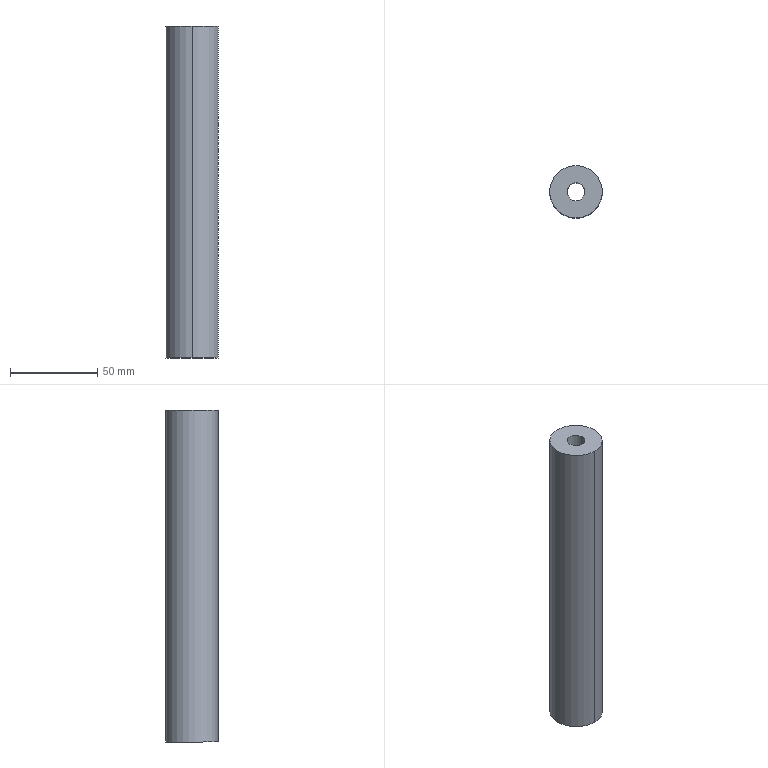Part | SolidWorks | features BaseBody 1 | 1 solid | 6 faces | box 30 x 30 x 190 mm | volume 118778 mm3 | cylinder 4 | plane 2 | commonest cylinder face diameters 10.2 x2 30 x2
STEP:
#1=CARTESIAN_POINT('',(5.1,0.,0.));
#2=VERTEX_POINT('',#1);
#3=CARTESIAN_POINT('',(-5.1,0.,0.));
#4=VERTEX_POINT('',#3);
#5=CARTESIAN_POINT('',(0.,0.,0.));
#6=DIRECTION('',(0.,0.,-1.));
#7=DIRECTION('',(1.,0.,0.));
#8=AXIS2_PLACEMENT_3D('',#5,#6,#7);
#9=CIRCLE('',#8,5.1);
#10=EDGE_CURVE('',#2,#4,#9,.T.);
#11=ORIENTED_EDGE('',*,*,#10,.T.);
#12=CARTESIAN_POINT('',(-5.1,0.,190.));
#13=VERTEX_POINT('',#12);
#14=CARTESIAN_POINT('',(-5.1,0.,0.));
#15=DIRECTION('',(0.,0.,1.));
#16=VECTOR('',#15,1000.);
#17=LINE('',#14,#16);
#18=EDGE_CURVE('',#4,#13,#17,.T.);
#19=ORIENTED_EDGE('',*,*,#18,.T.);
#20=CARTESIAN_POINT('',(5.1,0.,190.));
#21=VERTEX_POINT('',#20);
#22=CARTESIAN_POINT('',(0.,0.,190.));
#23=DIRECTION('',(0.,0.,1.));
#24=DIRECTION('',(1.,0.,0.));
#25=AXIS2_PLACEMENT_3D('',#22,#23,#24);
#26=CIRCLE('',#25,5.1);
#27=EDGE_CURVE('',#13,#21,#26,.T.);
#28=ORIENTED_EDGE('',*,*,#27,.T.);
#29=CARTESIAN_POINT('',(5.1,0.,0.));
#30=DIRECTION('',(0.,0.,1.));
#31=VECTOR('',#30,1000.);
#32=LINE('',#29,#31);
#33=EDGE_CURVE('',#2,#21,#32,.T.);
#34=ORIENTED_EDGE('',*,*,#33,.F.);
#35=EDGE_LOOP('',(#11,#19,#28,#34));
#36=FACE_OUTER_BOUND('',#35,.T.);
#37=CARTESIAN_POINT('',(0.,0.,0.));
#38=DIRECTION('',(0.,0.,1.));
#39=DIRECTION('',(1.,0.,0.));
#40=AXIS2_PLACEMENT_3D('',#37,#38,#39);
#41=CYLINDRICAL_SURFACE('',#40,5.1);
#42=ADVANCED_FACE('',(#36),#41,.F.);
#43=CARTESIAN_POINT('',(0.,-15.,190.));
#44=VERTEX_POINT('',#43);
#45=CARTESIAN_POINT('',(0.,15.,190.));
#46=VERTEX_POINT('',#45);
#47=CARTESIAN_POINT('',(0.,0.,190.));
#48=DIRECTION('',(0.,0.,1.));
#49=DIRECTION('',(0.,1.,0.));
#50=AXIS2_PLACEMENT_3D('',#47,#48,#49);
#51=CIRCLE('',#50,15.);
#52=EDGE_CURVE('',#44,#46,#51,.T.);
#53=ORIENTED_EDGE('',*,*,#52,.F.);
#54=CARTESIAN_POINT('',(0.,-15.,0.));
#55=VERTEX_POINT('',#54);
#56=CARTESIAN_POINT('',(0.,-15.,190.));
#57=DIRECTION('',(0.,0.,-1.));
#58=VECTOR('',#57,1000.);
#59=LINE('',#56,#58);
#60=EDGE_CURVE('',#44,#55,#59,.T.);
#61=ORIENTED_EDGE('',*,*,#60,.T.);
#62=CARTESIAN_POINT('',(0.,15.,0.));
#63=VERTEX_POINT('',#62);
#64=CARTESIAN_POINT('',(0.,0.,0.));
#65=DIRECTION('',(0.,0.,1.));
#66=DIRECTION('',(0.,1.,0.));
#67=AXIS2_PLACEMENT_3D('',#64,#65,#66);
#68=CIRCLE('',#67,15.);
#69=EDGE_CURVE('',#55,#63,#68,.T.);
#70=ORIENTED_EDGE('',*,*,#69,.T.);
#71=CARTESIAN_POINT('',(0.,15.,190.));
#72=DIRECTION('',(0.,0.,-1.));
#73=VECTOR('',#72,1000.);
#74=LINE('',#71,#73);
#75=EDGE_CURVE('',#46,#63,#74,.T.);
#76=ORIENTED_EDGE('',*,*,#75,.F.);
#77=EDGE_LOOP('',(#53,#61,#70,#76));
#78=FACE_OUTER_BOUND('',#77,.T.);
#79=CARTESIAN_POINT('',(0.,0.,190.));
#80=DIRECTION('',(0.,0.,-1.));
#81=DIRECTION('',(0.,1.,0.));
#82=AXIS2_PLACEMENT_3D('',#79,#80,#81);
#83=CYLINDRICAL_SURFACE('',#82,15.);
#84=ADVANCED_FACE('',(#78),#83,.T.);
#85=ORIENTED_EDGE('',*,*,#18,.F.);
#86=CARTESIAN_POINT('',(0.,0.,0.));
#87=DIRECTION('',(0.,0.,-1.));
#88=DIRECTION('',(1.,0.,0.));
#89=AXIS2_PLACEMENT_3D('',#86,#87,#88);
#90=CIRCLE('',#89,5.1);
#91=EDGE_CURVE('',#4,#2,#90,.T.);
#92=ORIENTED_EDGE('',*,*,#91,.T.);
#93=ORIENTED_EDGE('',*,*,#33,.T.);
#94=CARTESIAN_POINT('',(0.,0.,190.));
#95=DIRECTION('',(0.,0.,1.));
#96=DIRECTION('',(1.,0.,0.));
#97=AXIS2_PLACEMENT_3D('',#94,#95,#96);
#98=CIRCLE('',#97,5.1);
#99=EDGE_CURVE('',#21,#13,#98,.T.);
#100=ORIENTED_EDGE('',*,*,#99,.T.);
#101=EDGE_LOOP('',(#85,#92,#93,#100));
#102=FACE_OUTER_BOUND('',#101,.T.);
#103=CARTESIAN_POINT('',(0.,0.,0.));
#104=DIRECTION('',(0.,0.,1.));
#105=DIRECTION('',(1.,0.,0.));
#106=AXIS2_PLACEMENT_3D('',#103,#104,#105);
#107=CYLINDRICAL_SURFACE('',#106,5.1);
#108=ADVANCED_FACE('',(#102),#107,.F.);
#109=ORIENTED_EDGE('',*,*,#99,.F.);
#110=ORIENTED_EDGE('',*,*,#27,.F.);
#111=EDGE_LOOP('',(#109,#110));
#112=FACE_BOUND('',#111,.T.);
#113=CARTESIAN_POINT('',(0.,0.,190.));
#114=DIRECTION('',(0.,0.,1.));
#115=DIRECTION('',(0.,1.,0.));
#116=AXIS2_PLACEMENT_3D('',#113,#114,#115);
#117=CIRCLE('',#116,15.);
#118=EDGE_CURVE('',#46,#44,#117,.T.);
#119=ORIENTED_EDGE('',*,*,#118,.T.);
#120=ORIENTED_EDGE('',*,*,#52,.T.);
#121=EDGE_LOOP('',(#119,#120));
#122=FACE_OUTER_BOUND('',#121,.T.);
#123=CARTESIAN_POINT('',(-15.18,-15.18,190.));
#124=DIRECTION('',(0.,0.,1.));
#125=DIRECTION('',(1.,0.,0.));
#126=AXIS2_PLACEMENT_3D('',#123,#124,#125);
#127=PLANE('',#126);
#128=ADVANCED_FACE('',(#112,#122),#127,.T.);
#129=ORIENTED_EDGE('',*,*,#10,.F.);
#130=ORIENTED_EDGE('',*,*,#91,.F.);
#131=EDGE_LOOP('',(#129,#130));
#132=FACE_BOUND('',#131,.T.);
#133=CARTESIAN_POINT('',(0.,0.,0.));
#134=DIRECTION('',(0.,0.,1.));
#135=DIRECTION('',(0.,1.,0.));
#136=AXIS2_PLACEMENT_3D('',#133,#134,#135);
#137=CIRCLE('',#136,15.);
#138=EDGE_CURVE('',#63,#55,#137,.T.);
#139=ORIENTED_EDGE('',*,*,#138,.F.);
#140=ORIENTED_EDGE('',*,*,#69,.F.);
#141=EDGE_LOOP('',(#139,#140));
#142=FACE_OUTER_BOUND('',#141,.T.);
#143=CARTESIAN_POINT('',(-15.18,-15.18,0.));
#144=DIRECTION('',(0.,0.,1.));
#145=DIRECTION('',(1.,0.,0.));
#146=AXIS2_PLACEMENT_3D('',#143,#144,#145);
#147=PLANE('',#146);
#148=ADVANCED_FACE('',(#132,#142),#147,.F.);
#149=ORIENTED_EDGE('',*,*,#60,.F.);
#150=ORIENTED_EDGE('',*,*,#118,.F.);
#151=ORIENTED_EDGE('',*,*,#75,.T.);
#152=ORIENTED_EDGE('',*,*,#138,.T.);
#153=EDGE_LOOP('',(#149,#150,#151,#152));
#154=FACE_OUTER_BOUND('',#153,.T.);
#155=CARTESIAN_POINT('',(0.,0.,190.));
#156=DIRECTION('',(0.,0.,-1.));
#157=DIRECTION('',(0.,1.,0.));
#158=AXIS2_PLACEMENT_3D('',#155,#156,#157);
#159=CYLINDRICAL_SURFACE('',#158,15.);
#160=ADVANCED_FACE('',(#154),#159,.T.);
#161=CLOSED_SHELL('',(#42,#84,#108,#128,#148,#160));
#162=MANIFOLD_SOLID_BREP('',#161);
#163=CARTESIAN_POINT('',(0.,0.,0.));
#164=DIRECTION('',(0.,0.,1.));
#165=DIRECTION('',(1.,0.,0.));
#166=AXIS2_PLACEMENT_3D('',#163,#164,#165);
#167=(LENGTH_UNIT()NAMED_UNIT(*)SI_UNIT(.MILLI.,.METRE.));
#168=UNCERTAINTY_MEASURE_WITH_UNIT(LENGTH_MEASURE(0.00001),#167,'','');
#169=(NAMED_UNIT(*)PLANE_ANGLE_UNIT()SI_UNIT($,.RADIAN.));
#170=(NAMED_UNIT(*)SI_UNIT($,.STERADIAN.)SOLID_ANGLE_UNIT());
#171=(GEOMETRIC_REPRESENTATION_CONTEXT(3)GLOBAL_UNCERTAINTY_ASSIGNED_CONTEXT((#168))GLOBAL_UNIT_ASSIGNED_CONTEXT((#167,#169,#170))REPRESENTATION_CONTEXT('',''));
#172=ADVANCED_BREP_SHAPE_REPRESENTATION('',(#162,#166),#171);